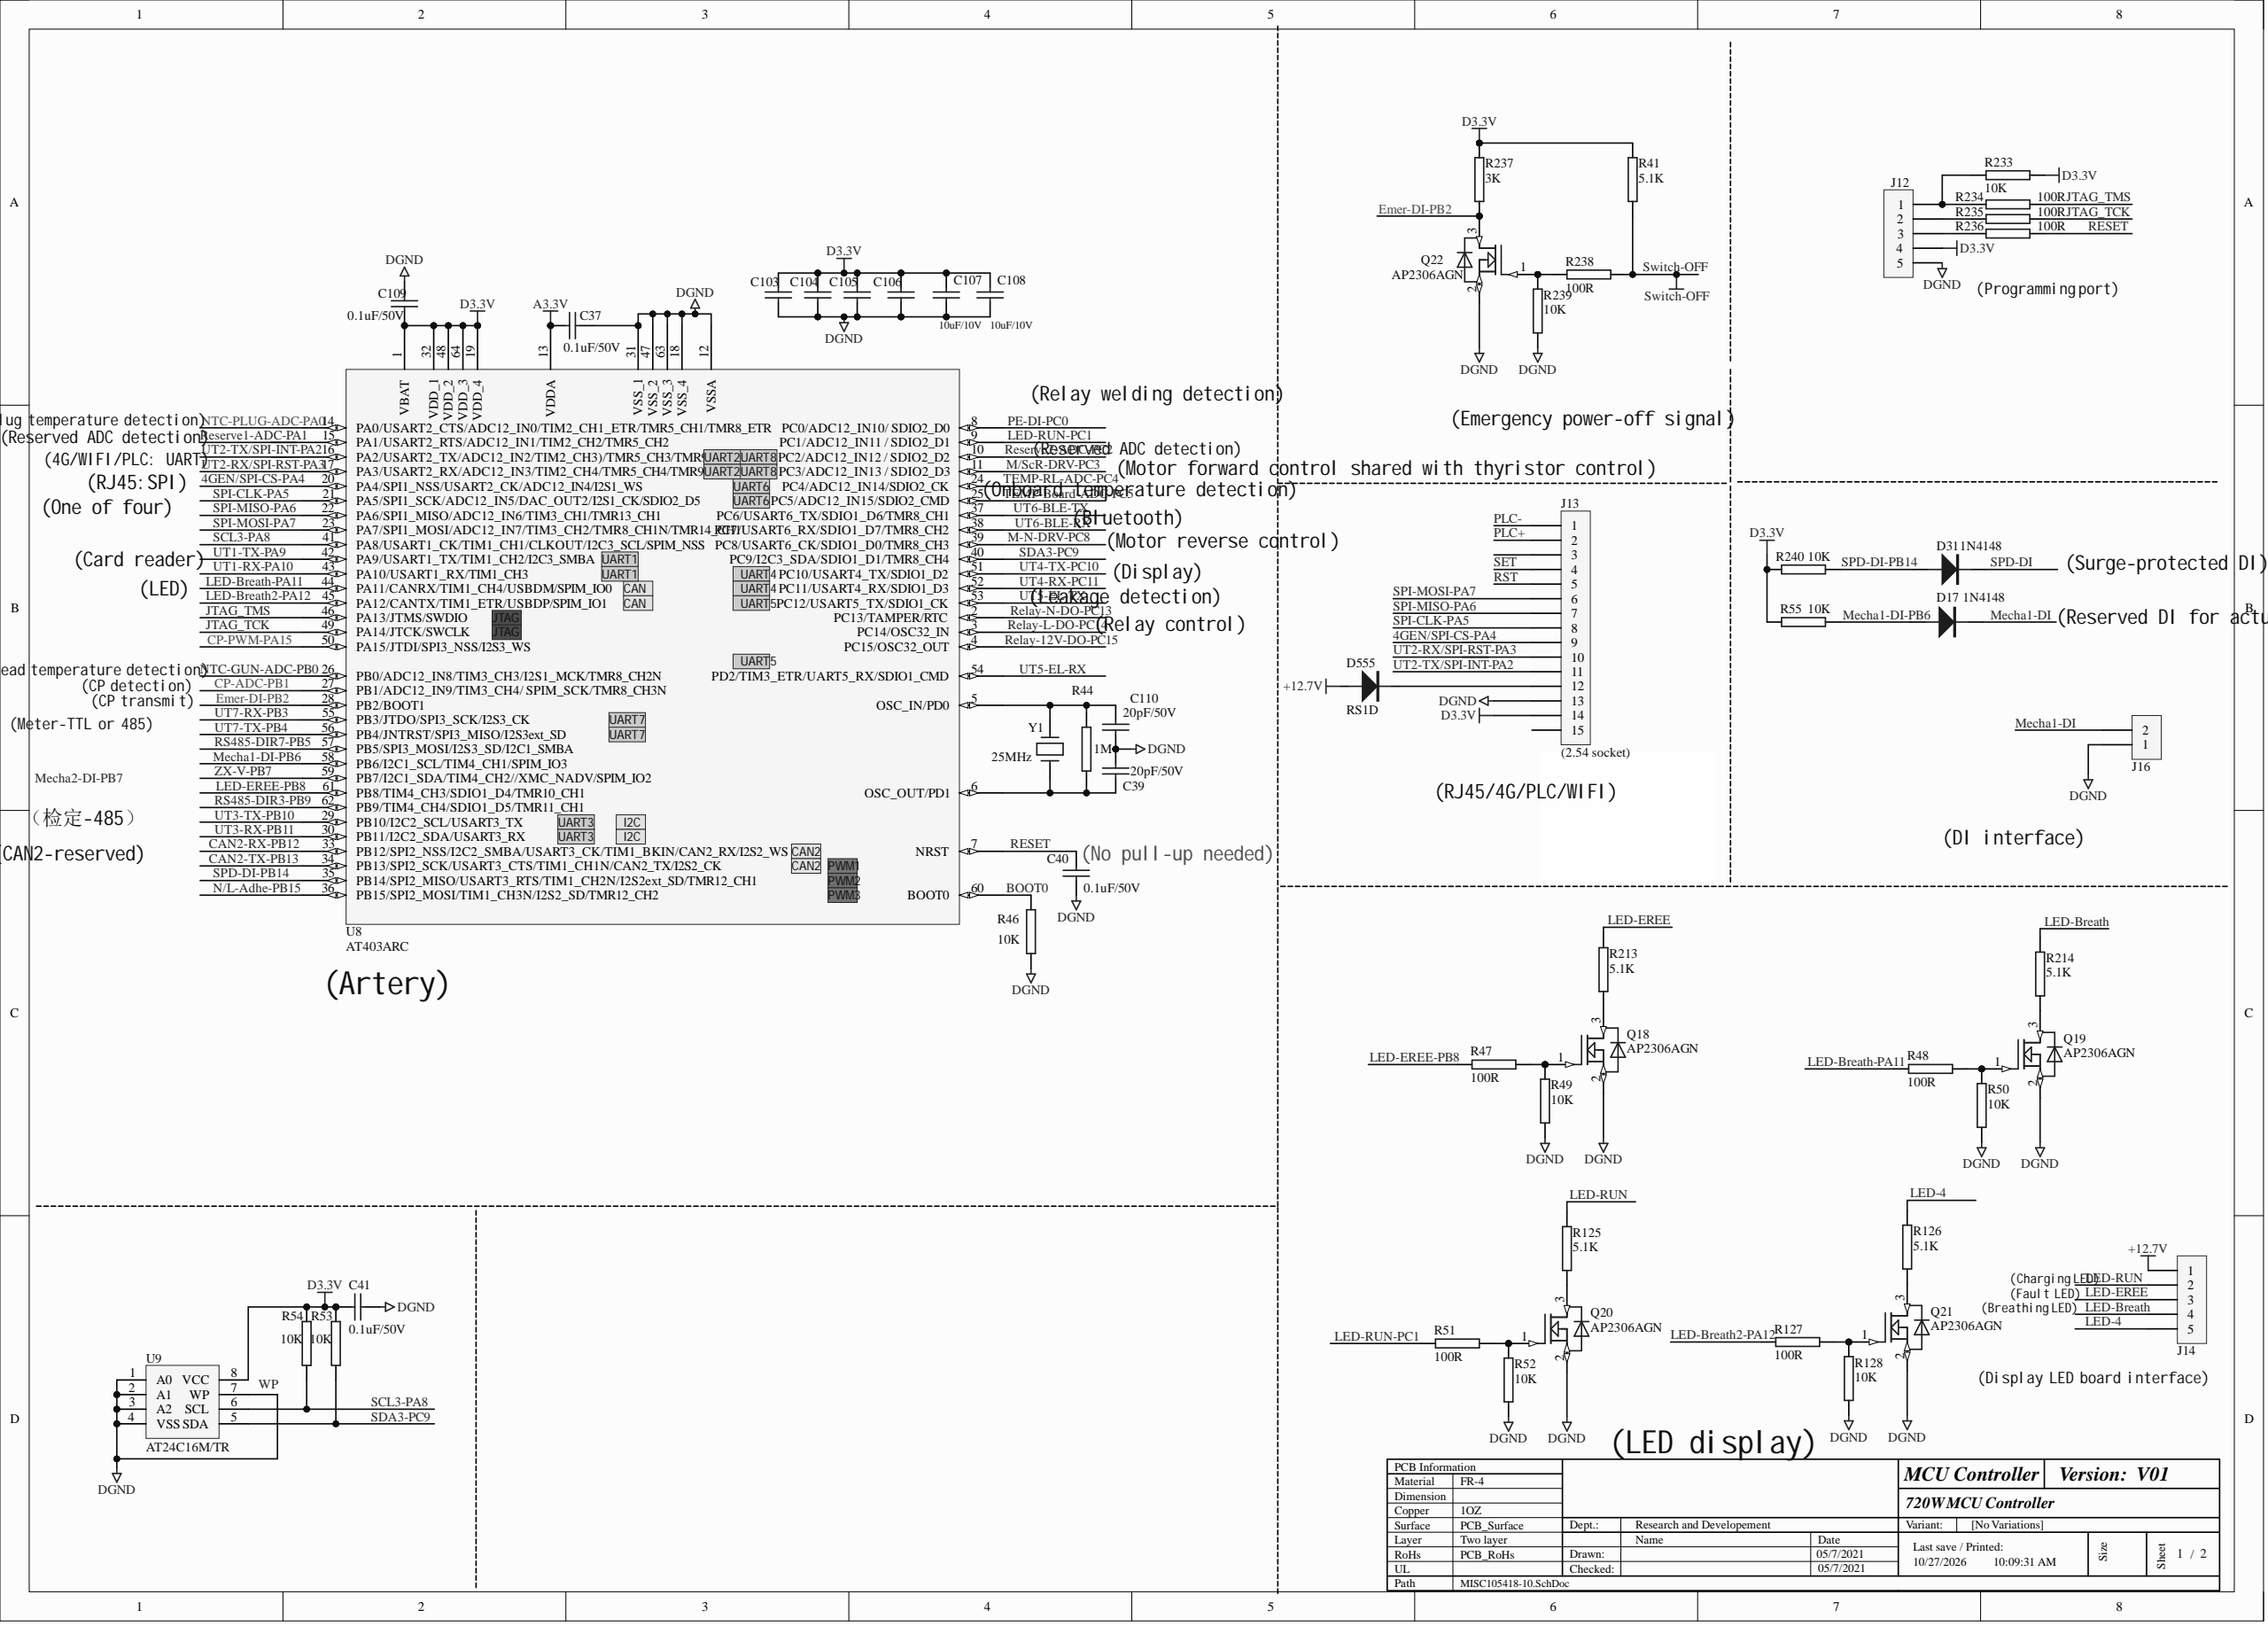Circuit board | Altium Designer | 455 parts | 280 nets | one sheet of the schematic
Parts on this sheet (reference | value | footprint):
C37 | 0.1uF/50V | C0603-T
C39 | 20pF/50V | C0603-T
C40 | 0.1uF/50V | C0603-T
C41 | 0.1uF/50V | C0603-T
C103 | 0.1uF/50V | C0603-T
C104 | 0.1uF/50V | C0603-T
C105 | 0.1uF/50V | C0603-T
C106 | 0.1uF/50V | C0603-T
C107 | 10uF/10V | C0805-T
C108 | 10uF/10V | C0805-T
C109 | 0.1uF/50V | C0603-T
C110 | 20pF/50V | C0603-T
D17 | 1N4148 | SOD-123-T
D555 | RS1D | SMA
J12 | CON5 | CON5-2.54
J13 | (2.54 socket) | P15-2.54
J14 | CON5 | CON5-2.54
J16 | CON2 | CON2-3.81
Q18 | AP2306AGN | SOT-23-T
Q19 | AP2306AGN | SOT-23-T
Q20 | AP2306AGN | SOT-23-T
Q21 | AP2306AGN | SOT-23-T
Q22 | AP2306AGN | SOT-23-T
R41 | 5.1K | R0603-T
R44 | 1M | R0603-T
R46 | 10K | R0603-T
R47 | 100R | R0603-T
R48 | 100R | R0603-T
R49 | 10K | R0603-T
R50 | 10K | R0603-T
R51 | 100R | R0603-T
R52 | 10K | R0603-T
R53 | 10K | R0603-T
R54 | 10K | R0603-T
R55 | 10K | R0603-T
R125 | 5.1K | R0603-T
R126 | 5.1K | R0603-T
R127 | 100R | R0603-T
R128 | 10K | R0603-T
R213 | 5.1K | R0603-T
R214 | 5.1K | R0603-T
R233 | 10K | R0603-T
R234 | 100R | R0603-T
R235 | 100R | R0603-T
R236 | 100R | R0603-T
R237 | 3K | R0603-T
R238 | 100R | R0603-T
R239 | 10K | R0603-T
R240 | 10K | R0603-T
U8 | AT403ARC | so-64-t1
U9 | AT24C16M/TR | SO-8-t
Y1 | 25MHz | SMD晶振（HC-49）
Nets of these parts (net: part-pin ...):
ZX-V-PB7: U8-59
UT7-TX-PB4: U8-56
UT7-RX-PB3: U8-55
UT6-BLE-TX: U8-37
UT6-BLE-RX: U8-38
UT5-EL-RX: U8-54
UT4-TX-PC10: U8-51
UT4-RX-PC11: U8-52
UT3-TX-PB10: U8-29
UT3-RX-PB11: U8-30
UT2-TX/SPI-\I\N\T\-PA2: J13-11 U8-16
UT2-RX/SPI-\R\S\T\-PA3: J13-10 U8-17
UT1-TX-PA9: U8-42
UT1-RX-PA10: U8-43
TEMP-RL-ADC-PC4: U8-24
TEMP-Board-ADC-PC5: U8-25
Switch-OFF: R41-2 R238-2
SPI-MOSI-PA7: J13-6 U8-23
SPI-MISO-PA6: J13-7 U8-22
SPI-CLK-PA5: J13-8 U8-21
SPD-DI-PB14: R240-2 U8-35
SDA3-PC9: R53-2 U9-5 U8-40
SCL3-PA8: R54-2 U9-6 U8-41
RS485-DIR3-PB9: U8-62
RESET: C40-1 R236-2 U8-7
Reserve2-ADC-PC2: U8-10
Reserve1-ADC-PA1: U8-15
Relay-N-DO-PC13: U8-2
Relay-L-DO-PC14: U8-3
Relay-12V-DO-PC15: U8-4
PLC-: J13-1
PLC+: J13-2
PE-DI-PC0: U8-8
NTC-PLUG-ADC-PA0: U8-14
NTC-GUN-ADC-PB0: U8-26
NetQ22_1: Q22-1 R238-1 R239-1
NetQ21_3: Q21-3 R126-2
NetQ21_1: Q21-1 R127-1 R128-1
NetQ20_3: Q20-3 R125-2
NetQ20_1: Q20-1 R51-1 R52-1
NetQ19_3: Q19-3 R214-2
NetQ19_1: Q19-1 R48-1 R50-1
NetQ18_3: Q18-3 R213-2
NetQ18_1: Q18-1 R47-1 R49-1
NetJ12_3: J12-3 R236-1
NetJ12_2: J12-2 R235-1
NetJ12_1: J12-1 R233-2 R234-1
NetD555_2: D555-2 J13-12
NetC110_1: C110-1 R44-1 Y1-2 U8-5
NetC39_2: C39-2 R44-2 Y1-1 U8-6
N/L-Adhe-PB15: U8-36
Mecha1-DI-PB6: D17-1 R55-2 U8-58
Mecha1-DI: D17-2 J16-2
M/ScR-DRV-PC3: U8-11
M-N-DRV-PC8: U8-39
LED-RUN-PC1: R51-2 U8-9
LED-RUN: J14-2 R125-1
LED-EREE-PB8: R47-2 U8-61
LED-EREE: J14-3 R213-1
LED-Breath-PA11: R48-2 U8-44
LED-Breath2-PA12: R127-2 U8-45
LED-Breath: J14-4 R214-1
LED-4: J14-5 R126-1
JTAG_TMS: R234-2 U8-46
JTAG_TCK: R235-2 U8-49
Emer-DI-PB2: Q22-3 R237-2 U8-28
D3.3V: C41-2 C103-1 C104-1 C105-1 C106-1 C107-1 C108-1 C109-2 J12-4 J13-14 R41-1 R53-1 R54-1 R55-1 R233-1 R237-1 R240-1 U9-8 U8-1 U8-19 U8-32 U8-48 U8-64
CP-PWM-PA15: U8-50
CAN2-TX-PB13: U8-34
CAN2-RX-PB12: U8-33
BOOT0: R46-1 U8-60
A3.3V: C37-2 U8-13
-: C37-1 C39-1 C40-2 C41-1 C103-2 C104-2 C105-2 C106-2 C107-2 C108-2 C109-1 C110-2 J12-5 J13-13 J16-1 Q18-2 Q19-2 Q20-2 Q21-2 Q22-2 R46-2 R49-2 R50-2 R52-2 R128-2 R239-2 U9-1 U9-2 U9-3 U9-4 U9-7 U8-12 U8-18 U8-31 U8-47 U8-63
+12.7V: D555-1 J14-1
4GEN/SPI-CS-PA4: J13-9 U8-20